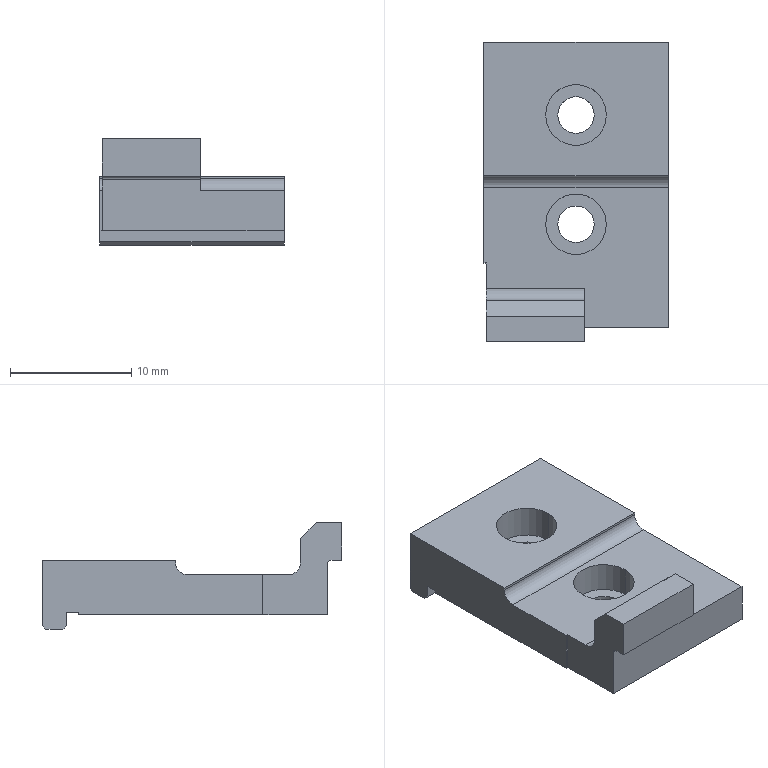Part | NX | 1 solid | 35 faces | box 15.2 x 24.7 x 8.8 mm | volume 1393 mm3 | plane 24 | cylinder 11 | commonest cylinder face diameters 3 x4 5 x4 2 x2 0.6 x1
STEP:
#1=CARTESIAN_POINT('',(0.2,6.5,-4.5));
#2=VERTEX_POINT('',#1);
#3=CARTESIAN_POINT('',(0.,6.5,-4.5));
#4=VERTEX_POINT('',#3);
#5=CARTESIAN_POINT('',(0.,6.5,-4.5));
#6=DIRECTION('',(-1.,0.,0.));
#7=VECTOR('',#6,1000.);
#8=LINE('',#5,#7);
#9=EDGE_CURVE('',#2,#4,#8,.T.);
#10=ORIENTED_EDGE('',*,*,#9,.T.);
#11=CARTESIAN_POINT('',(0.,21.7,-4.5));
#12=VERTEX_POINT('',#11);
#13=CARTESIAN_POINT('',(0.,0.,-4.5));
#14=DIRECTION('',(0.,-1.,0.));
#15=VECTOR('',#14,1000.);
#16=LINE('',#13,#15);
#17=EDGE_CURVE('',#12,#4,#16,.T.);
#18=ORIENTED_EDGE('',*,*,#17,.F.);
#19=CARTESIAN_POINT('',(15.2,21.7,-4.5));
#20=VERTEX_POINT('',#19);
#21=CARTESIAN_POINT('',(0.,21.7,-4.5));
#22=DIRECTION('',(1.,0.,0.));
#23=VECTOR('',#22,1000.);
#24=LINE('',#21,#23);
#25=EDGE_CURVE('',#12,#20,#24,.T.);
#26=ORIENTED_EDGE('',*,*,#25,.T.);
#27=CARTESIAN_POINT('',(15.2,1.2,-4.5));
#28=VERTEX_POINT('',#27);
#29=CARTESIAN_POINT('',(15.2,0.,-4.5));
#30=DIRECTION('',(0.,1.,0.));
#31=VECTOR('',#30,1000.);
#32=LINE('',#29,#31);
#33=EDGE_CURVE('',#28,#20,#32,.T.);
#34=ORIENTED_EDGE('',*,*,#33,.F.);
#35=CARTESIAN_POINT('',(0.2,1.2,-4.5));
#36=VERTEX_POINT('',#35);
#37=CARTESIAN_POINT('',(0.,1.2,-4.5));
#38=DIRECTION('',(-1.,0.,0.));
#39=VECTOR('',#38,1000.);
#40=LINE('',#37,#39);
#41=EDGE_CURVE('',#28,#36,#40,.T.);
#42=ORIENTED_EDGE('',*,*,#41,.T.);
#43=CARTESIAN_POINT('',(0.2,0.,-4.5));
#44=DIRECTION('',(0.,1.,0.));
#45=VECTOR('',#44,1000.);
#46=LINE('',#43,#45);
#47=EDGE_CURVE('',#36,#2,#46,.T.);
#48=ORIENTED_EDGE('',*,*,#47,.T.);
#49=EDGE_LOOP('',(#10,#18,#26,#34,#42,#48));
#50=FACE_BOUND('',#49,.T.);
#51=CARTESIAN_POINT('',(9.1,9.7,-4.5));
#52=VERTEX_POINT('',#51);
#53=CARTESIAN_POINT('',(6.1,9.7,-4.5));
#54=VERTEX_POINT('',#53);
#55=CARTESIAN_POINT('',(7.6,9.7,-4.5));
#56=DIRECTION('',(0.,0.,1.));
#57=DIRECTION('',(-1.,0.,0.));
#58=AXIS2_PLACEMENT_3D('',#55,#56,#57);
#59=CIRCLE('',#58,1.5);
#60=EDGE_CURVE('',#52,#54,#59,.T.);
#61=ORIENTED_EDGE('',*,*,#60,.T.);
#62=CARTESIAN_POINT('',(7.6,9.7,-4.5));
#63=DIRECTION('',(0.,0.,1.));
#64=DIRECTION('',(-1.,0.,0.));
#65=AXIS2_PLACEMENT_3D('',#62,#63,#64);
#66=CIRCLE('',#65,1.5);
#67=EDGE_CURVE('',#54,#52,#66,.T.);
#68=ORIENTED_EDGE('',*,*,#67,.T.);
#69=EDGE_LOOP('',(#61,#68));
#70=FACE_BOUND('',#69,.T.);
#71=CARTESIAN_POINT('',(6.1,18.7,-4.5));
#72=VERTEX_POINT('',#71);
#73=CARTESIAN_POINT('',(9.1,18.7,-4.5));
#74=VERTEX_POINT('',#73);
#75=CARTESIAN_POINT('',(7.6,18.7,-4.5));
#76=DIRECTION('',(0.,0.,1.));
#77=DIRECTION('',(-1.,0.,0.));
#78=AXIS2_PLACEMENT_3D('',#75,#76,#77);
#79=CIRCLE('',#78,1.5);
#80=EDGE_CURVE('',#72,#74,#79,.T.);
#81=ORIENTED_EDGE('',*,*,#80,.T.);
#82=CARTESIAN_POINT('',(7.6,18.7,-4.5));
#83=DIRECTION('',(0.,0.,1.));
#84=DIRECTION('',(-1.,0.,0.));
#85=AXIS2_PLACEMENT_3D('',#82,#83,#84);
#86=CIRCLE('',#85,1.5);
#87=EDGE_CURVE('',#74,#72,#86,.T.);
#88=ORIENTED_EDGE('',*,*,#87,.T.);
#89=EDGE_LOOP('',(#81,#88));
#90=FACE_BOUND('',#89,.T.);
#91=CARTESIAN_POINT('',(0.,0.,-4.5));
#92=DIRECTION('',(0.,0.,1.));
#93=DIRECTION('',(1.,0.,0.));
#94=AXIS2_PLACEMENT_3D('',#91,#92,#93);
#95=PLANE('',#94);
#96=ADVANCED_FACE('',(#50,#70,#90),#95,.F.);
#97=CARTESIAN_POINT('',(0.2,4.4,-1.2));
#98=VERTEX_POINT('',#97);
#99=CARTESIAN_POINT('',(0.2,6.5,-1.2));
#100=VERTEX_POINT('',#99);
#101=CARTESIAN_POINT('',(0.2,0.,-1.2));
#102=DIRECTION('',(0.,1.,0.));
#103=VECTOR('',#102,1000.);
#104=LINE('',#101,#103);
#105=EDGE_CURVE('',#98,#100,#104,.T.);
#106=ORIENTED_EDGE('',*,*,#105,.T.);
#107=CARTESIAN_POINT('',(0.2,6.5,0.));
#108=DIRECTION('',(0.,0.,-1.));
#109=VECTOR('',#108,1000.);
#110=LINE('',#107,#109);
#111=EDGE_CURVE('',#100,#2,#110,.T.);
#112=ORIENTED_EDGE('',*,*,#111,.T.);
#113=ORIENTED_EDGE('',*,*,#47,.F.);
#114=CARTESIAN_POINT('',(0.2,1.2,-0.3));
#115=VERTEX_POINT('',#114);
#116=CARTESIAN_POINT('',(0.2,1.2,0.));
#117=DIRECTION('',(0.,0.,-1.));
#118=VECTOR('',#117,1000.);
#119=LINE('',#116,#118);
#120=EDGE_CURVE('',#115,#36,#119,.T.);
#121=ORIENTED_EDGE('',*,*,#120,.F.);
#122=CARTESIAN_POINT('',(0.2,0.9,0.));
#123=VERTEX_POINT('',#122);
#124=CARTESIAN_POINT('',(0.2,0.9,-0.3));
#125=DIRECTION('',(-1.,0.,0.));
#126=DIRECTION('',(0.,0.,1.));
#127=AXIS2_PLACEMENT_3D('',#124,#125,#126);
#128=CIRCLE('',#127,0.3);
#129=EDGE_CURVE('',#123,#115,#128,.T.);
#130=ORIENTED_EDGE('',*,*,#129,.F.);
#131=CARTESIAN_POINT('',(0.2,0.,0.));
#132=VERTEX_POINT('',#131);
#133=CARTESIAN_POINT('',(0.2,0.,0.));
#134=DIRECTION('',(0.,1.,0.));
#135=VECTOR('',#134,1000.);
#136=LINE('',#133,#135);
#137=EDGE_CURVE('',#132,#123,#136,.T.);
#138=ORIENTED_EDGE('',*,*,#137,.F.);
#139=CARTESIAN_POINT('',(0.2,0.,3.1));
#140=VERTEX_POINT('',#139);
#141=CARTESIAN_POINT('',(0.2,0.,0.));
#142=DIRECTION('',(0.,0.,1.));
#143=VECTOR('',#142,1000.);
#144=LINE('',#141,#143);
#145=EDGE_CURVE('',#132,#140,#144,.T.);
#146=ORIENTED_EDGE('',*,*,#145,.T.);
#147=CARTESIAN_POINT('',(0.2,2.1,3.1));
#148=VERTEX_POINT('',#147);
#149=CARTESIAN_POINT('',(0.2,0.,3.1));
#150=DIRECTION('',(0.,1.,0.));
#151=VECTOR('',#150,1000.);
#152=LINE('',#149,#151);
#153=EDGE_CURVE('',#140,#148,#152,.T.);
#154=ORIENTED_EDGE('',*,*,#153,.T.);
#155=CARTESIAN_POINT('',(0.2,3.4,1.8));
#156=VERTEX_POINT('',#155);
#157=CARTESIAN_POINT('',(0.2,5.2,0.));
#158=DIRECTION('',(0.,-0.7071,0.7071));
#159=VECTOR('',#158,1000.);
#160=LINE('',#157,#159);
#161=EDGE_CURVE('',#156,#148,#160,.T.);
#162=ORIENTED_EDGE('',*,*,#161,.F.);
#163=CARTESIAN_POINT('',(0.2,3.4,-0.2));
#164=VERTEX_POINT('',#163);
#165=CARTESIAN_POINT('',(0.2,3.4,0.));
#166=DIRECTION('',(0.,0.,1.));
#167=VECTOR('',#166,1000.);
#168=LINE('',#165,#167);
#169=EDGE_CURVE('',#164,#156,#168,.T.);
#170=ORIENTED_EDGE('',*,*,#169,.F.);
#171=CARTESIAN_POINT('',(0.2,4.4,-0.2));
#172=DIRECTION('',(-1.,0.,0.));
#173=DIRECTION('',(0.,1.,0.));
#174=AXIS2_PLACEMENT_3D('',#171,#172,#173);
#175=CIRCLE('',#174,1.);
#176=EDGE_CURVE('',#98,#164,#175,.T.);
#177=ORIENTED_EDGE('',*,*,#176,.F.);
#178=EDGE_LOOP('',(#106,#112,#113,#121,#130,#138,#146,#154,#162,#170,#177));
#179=FACE_BOUND('',#178,.T.);
#180=CARTESIAN_POINT('',(0.2,6.5,-2.));
#181=DIRECTION('',(1.,0.,0.));
#182=DIRECTION('',(0.,1.,0.));
#183=AXIS2_PLACEMENT_3D('',#180,#181,#182);
#184=PLANE('',#183);
#185=ADVANCED_FACE('',(#179),#184,.F.);
#186=ORIENTED_EDGE('',*,*,#9,.F.);
#187=ORIENTED_EDGE('',*,*,#111,.F.);
#188=CARTESIAN_POINT('',(0.,6.5,-1.2));
#189=VERTEX_POINT('',#188);
#190=CARTESIAN_POINT('',(0.,6.5,-1.2));
#191=DIRECTION('',(1.,0.,0.));
#192=VECTOR('',#191,1000.);
#193=LINE('',#190,#192);
#194=EDGE_CURVE('',#189,#100,#193,.T.);
#195=ORIENTED_EDGE('',*,*,#194,.F.);
#196=CARTESIAN_POINT('',(0.,6.5,0.));
#197=DIRECTION('',(0.,0.,1.));
#198=VECTOR('',#197,1000.);
#199=LINE('',#196,#198);
#200=EDGE_CURVE('',#4,#189,#199,.T.);
#201=ORIENTED_EDGE('',*,*,#200,.F.);
#202=EDGE_LOOP('',(#186,#187,#195,#201));
#203=FACE_BOUND('',#202,.T.);
#204=CARTESIAN_POINT('',(0.,6.5,-2.));
#205=DIRECTION('',(0.,1.,0.));
#206=DIRECTION('',(1.,0.,0.));
#207=AXIS2_PLACEMENT_3D('',#204,#205,#206);
#208=PLANE('',#207);
#209=ADVANCED_FACE('',(#203),#208,.F.);
#210=CARTESIAN_POINT('',(10.1,18.7,-2.7));
#211=VERTEX_POINT('',#210);
#212=CARTESIAN_POINT('',(5.1,18.7,-2.7));
#213=VERTEX_POINT('',#212);
#214=CARTESIAN_POINT('',(7.6,18.7,-2.7));
#215=DIRECTION('',(0.,0.,1.));
#216=DIRECTION('',(-1.,0.,0.));
#217=AXIS2_PLACEMENT_3D('',#214,#215,#216);
#218=CIRCLE('',#217,2.5);
#219=EDGE_CURVE('',#211,#213,#218,.T.);
#220=ORIENTED_EDGE('',*,*,#219,.T.);
#221=CARTESIAN_POINT('',(7.6,18.7,-2.7));
#222=DIRECTION('',(0.,0.,1.));
#223=DIRECTION('',(-1.,0.,0.));
#224=AXIS2_PLACEMENT_3D('',#221,#222,#223);
#225=CIRCLE('',#224,2.5);
#226=EDGE_CURVE('',#213,#211,#225,.T.);
#227=ORIENTED_EDGE('',*,*,#226,.T.);
#228=EDGE_LOOP('',(#220,#227));
#229=FACE_BOUND('',#228,.T.);
#230=CARTESIAN_POINT('',(6.1,18.7,-2.7));
#231=VERTEX_POINT('',#230);
#232=CARTESIAN_POINT('',(9.1,18.7,-2.7));
#233=VERTEX_POINT('',#232);
#234=CARTESIAN_POINT('',(7.6,18.7,-2.7));
#235=DIRECTION('',(0.,0.,1.));
#236=DIRECTION('',(-1.,0.,0.));
#237=AXIS2_PLACEMENT_3D('',#234,#235,#236);
#238=CIRCLE('',#237,1.5);
#239=EDGE_CURVE('',#231,#233,#238,.T.);
#240=ORIENTED_EDGE('',*,*,#239,.F.);
#241=CARTESIAN_POINT('',(7.6,18.7,-2.7));
#242=DIRECTION('',(0.,0.,1.));
#243=DIRECTION('',(-1.,0.,0.));
#244=AXIS2_PLACEMENT_3D('',#241,#242,#243);
#245=CIRCLE('',#244,1.5);
#246=EDGE_CURVE('',#233,#231,#245,.T.);
#247=ORIENTED_EDGE('',*,*,#246,.F.);
#248=EDGE_LOOP('',(#240,#247));
#249=FACE_BOUND('',#248,.T.);
#250=CARTESIAN_POINT('',(6.068,11.447,-2.7));
#251=DIRECTION('',(0.,0.,1.));
#252=DIRECTION('',(1.,0.,0.));
#253=AXIS2_PLACEMENT_3D('',#250,#251,#252);
#254=PLANE('',#253);
#255=ADVANCED_FACE('',(#229,#249),#254,.T.);
#256=CARTESIAN_POINT('',(0.,13.7,-0.2));
#257=VERTEX_POINT('',#256);
#258=CARTESIAN_POINT('',(0.,13.7,0.));
#259=VERTEX_POINT('',#258);
#260=CARTESIAN_POINT('',(0.,13.7,0.));
#261=DIRECTION('',(0.,0.,1.));
#262=VECTOR('',#261,1000.);
#263=LINE('',#260,#262);
#264=EDGE_CURVE('',#257,#259,#263,.T.);
#265=ORIENTED_EDGE('',*,*,#264,.T.);
#266=CARTESIAN_POINT('',(0.,24.7,0.));
#267=VERTEX_POINT('',#266);
#268=CARTESIAN_POINT('',(0.,0.,0.));
#269=DIRECTION('',(0.,-1.,0.));
#270=VECTOR('',#269,1000.);
#271=LINE('',#268,#270);
#272=EDGE_CURVE('',#267,#259,#271,.T.);
#273=ORIENTED_EDGE('',*,*,#272,.F.);
#274=CARTESIAN_POINT('',(0.,24.7,-5.4));
#275=VERTEX_POINT('',#274);
#276=CARTESIAN_POINT('',(0.,24.7,0.));
#277=DIRECTION('',(0.,0.,-1.));
#278=VECTOR('',#277,1000.);
#279=LINE('',#276,#278);
#280=EDGE_CURVE('',#267,#275,#279,.T.);
#281=ORIENTED_EDGE('',*,*,#280,.T.);
#282=CARTESIAN_POINT('',(0.,24.4,-5.7));
#283=VERTEX_POINT('',#282);
#284=CARTESIAN_POINT('',(0.,0.,-30.1));
#285=DIRECTION('',(0.,-0.7071,-0.7071));
#286=VECTOR('',#285,1000.);
#287=LINE('',#284,#286);
#288=EDGE_CURVE('',#275,#283,#287,.T.);
#289=ORIENTED_EDGE('',*,*,#288,.T.);
#290=CARTESIAN_POINT('',(0.,23.,-5.7));
#291=VERTEX_POINT('',#290);
#292=CARTESIAN_POINT('',(0.,0.,-5.7));
#293=DIRECTION('',(0.,1.,0.));
#294=VECTOR('',#293,1000.);
#295=LINE('',#292,#294);
#296=EDGE_CURVE('',#291,#283,#295,.T.);
#297=ORIENTED_EDGE('',*,*,#296,.F.);
#298=CARTESIAN_POINT('',(0.,22.7,-5.4));
#299=VERTEX_POINT('',#298);
#300=CARTESIAN_POINT('',(0.,0.,17.3));
#301=DIRECTION('',(0.,-0.7071,0.7071));
#302=VECTOR('',#301,1000.);
#303=LINE('',#300,#302);
#304=EDGE_CURVE('',#291,#299,#303,.T.);
#305=ORIENTED_EDGE('',*,*,#304,.T.);
#306=CARTESIAN_POINT('',(0.,22.7,-4.3));
#307=VERTEX_POINT('',#306);
#308=CARTESIAN_POINT('',(0.,22.7,0.));
#309=DIRECTION('',(0.,0.,-1.));
#310=VECTOR('',#309,1000.);
#311=LINE('',#308,#310);
#312=EDGE_CURVE('',#307,#299,#311,.T.);
#313=ORIENTED_EDGE('',*,*,#312,.F.);
#314=CARTESIAN_POINT('',(0.,21.7,-4.3));
#315=VERTEX_POINT('',#314);
#316=CARTESIAN_POINT('',(0.,0.,-4.3));
#317=DIRECTION('',(0.,-1.,0.));
#318=VECTOR('',#317,1000.);
#319=LINE('',#316,#318);
#320=EDGE_CURVE('',#307,#315,#319,.T.);
#321=ORIENTED_EDGE('',*,*,#320,.T.);
#322=CARTESIAN_POINT('',(0.,21.7,0.));
#323=DIRECTION('',(0.,0.,-1.));
#324=VECTOR('',#323,1000.);
#325=LINE('',#322,#324);
#326=EDGE_CURVE('',#315,#12,#325,.T.);
#327=ORIENTED_EDGE('',*,*,#326,.T.);
#328=ORIENTED_EDGE('',*,*,#17,.T.);
#329=ORIENTED_EDGE('',*,*,#200,.T.);
#330=CARTESIAN_POINT('',(0.,12.7,-1.2));
#331=VERTEX_POINT('',#330);
#332=CARTESIAN_POINT('',(0.,0.,-1.2));
#333=DIRECTION('',(0.,-1.,0.));
#334=VECTOR('',#333,1000.);
#335=LINE('',#332,#334);
#336=EDGE_CURVE('',#331,#189,#335,.T.);
#337=ORIENTED_EDGE('',*,*,#336,.F.);
#338=CARTESIAN_POINT('',(0.,12.7,-0.2));
#339=DIRECTION('',(-1.,0.,0.));
#340=DIRECTION('',(0.,1.,0.));
#341=AXIS2_PLACEMENT_3D('',#338,#339,#340);
#342=CIRCLE('',#341,1.);
#343=EDGE_CURVE('',#257,#331,#342,.T.);
#344=ORIENTED_EDGE('',*,*,#343,.F.);
#345=EDGE_LOOP('',(#265,#273,#281,#289,#297,#305,#313,#321,#327,#328,#329,#337,#344));
#346=FACE_BOUND('',#345,.T.);
#347=CARTESIAN_POINT('',(0.,24.7,0.));
#348=DIRECTION('',(-1.,0.,0.));
#349=DIRECTION('',(0.,0.,1.));
#350=AXIS2_PLACEMENT_3D('',#347,#348,#349);
#351=PLANE('',#350);
#352=ADVANCED_FACE('',(#346),#351,.T.);
#353=CARTESIAN_POINT('',(8.3,4.4,-1.2));
#354=VERTEX_POINT('',#353);
#355=CARTESIAN_POINT('',(0.,4.4,-1.2));
#356=DIRECTION('',(-1.,0.,0.));
#357=VECTOR('',#356,1000.);
#358=LINE('',#355,#357);
#359=EDGE_CURVE('',#354,#98,#358,.T.);
#360=ORIENTED_EDGE('',*,*,#359,.T.);
#361=ORIENTED_EDGE('',*,*,#176,.T.);
#362=CARTESIAN_POINT('',(8.3,3.4,-0.2));
#363=VERTEX_POINT('',#362);
#364=CARTESIAN_POINT('',(0.,3.4,-0.2));
#365=DIRECTION('',(-1.,0.,0.));
#366=VECTOR('',#365,1000.);
#367=LINE('',#364,#366);
#368=EDGE_CURVE('',#363,#164,#367,.T.);
#369=ORIENTED_EDGE('',*,*,#368,.F.);
#370=CARTESIAN_POINT('',(8.3,4.4,-0.2));
#371=DIRECTION('',(-1.,0.,0.));
#372=DIRECTION('',(0.,1.,0.));
#373=AXIS2_PLACEMENT_3D('',#370,#371,#372);
#374=CIRCLE('',#373,1.);
#375=EDGE_CURVE('',#354,#363,#374,.T.);
#376=ORIENTED_EDGE('',*,*,#375,.F.);
#377=EDGE_LOOP('',(#360,#361,#369,#376));
#378=FACE_BOUND('',#377,.T.);
#379=CARTESIAN_POINT('',(0.,4.4,-0.2));
#380=DIRECTION('',(-1.,0.,0.));
#381=DIRECTION('',(0.,1.,0.));
#382=AXIS2_PLACEMENT_3D('',#379,#380,#381);
#383=CYLINDRICAL_SURFACE('',#382,1.);
#384=ADVANCED_FACE('',(#378),#383,.F.);
#385=ORIENTED_EDGE('',*,*,#264,.F.);
#386=CARTESIAN_POINT('',(15.2,13.7,-0.2));
#387=VERTEX_POINT('',#386);
#388=CARTESIAN_POINT('',(0.,13.7,-0.2));
#389=DIRECTION('',(-1.,0.,0.));
#390=VECTOR('',#389,1000.);
#391=LINE('',#388,#390);
#392=EDGE_CURVE('',#387,#257,#391,.T.);
#393=ORIENTED_EDGE('',*,*,#392,.F.);
#394=CARTESIAN_POINT('',(15.2,13.7,0.));
#395=VERTEX_POINT('',#394);
#396=CARTESIAN_POINT('',(15.2,13.7,0.));
#397=DIRECTION('',(0.,0.,-1.));
#398=VECTOR('',#397,1000.);
#399=LINE('',#396,#398);
#400=EDGE_CURVE('',#395,#387,#399,.T.);
#401=ORIENTED_EDGE('',*,*,#400,.F.);
#402=CARTESIAN_POINT('',(0.,13.7,0.));
#403=DIRECTION('',(-1.,0.,0.));
#404=VECTOR('',#403,1000.);
#405=LINE('',#402,#404);
#406=EDGE_CURVE('',#395,#259,#405,.T.);
#407=ORIENTED_EDGE('',*,*,#406,.T.);
#408=EDGE_LOOP('',(#385,#393,#401,#407));
#409=FACE_BOUND('',#408,.T.);
#410=CARTESIAN_POINT('',(15.2,13.7,-1.));
#411=DIRECTION('',(0.,1.,0.));
#412=DIRECTION('',(1.,0.,0.));
#413=AXIS2_PLACEMENT_3D('',#410,#411,#412);
#414=PLANE('',#413);
#415=ADVANCED_FACE('',(#409),#414,.F.);
#416=ORIENTED_EDGE('',*,*,#120,.T.);
#417=ORIENTED_EDGE('',*,*,#41,.F.);
#418=CARTESIAN_POINT('',(15.2,1.2,-1.2));
#419=VERTEX_POINT('',#418);
#420=CARTESIAN_POINT('',(15.2,1.2,0.));
#421=DIRECTION('',(0.,0.,-1.));
#422=VECTOR('',#421,1000.);
#423=LINE('',#420,#422);
#424=EDGE_CURVE('',#419,#28,#423,.T.);
#425=ORIENTED_EDGE('',*,*,#424,.F.);
#426=CARTESIAN_POINT('',(8.3,1.2,-1.2));
#427=VERTEX_POINT('',#426);
#428=CARTESIAN_POINT('',(0.,1.2,-1.2));
#429=DIRECTION('',(1.,0.,0.));
#430=VECTOR('',#429,1000.);
#431=LINE('',#428,#430);
#432=EDGE_CURVE('',#427,#419,#431,.T.);
#433=ORIENTED_EDGE('',*,*,#432,.F.);
#434=CARTESIAN_POINT('',(8.3,1.2,-0.3));
#435=VERTEX_POINT('',#434);
#436=CARTESIAN_POINT('',(8.3,1.2,0.));
#437=DIRECTION('',(0.,0.,1.));
#438=VECTOR('',#437,1000.);
#439=LINE('',#436,#438);
#440=EDGE_CURVE('',#427,#435,#439,.T.);
#441=ORIENTED_EDGE('',*,*,#440,.T.);
#442=CARTESIAN_POINT('',(15.289,1.2,-0.3));
#443=DIRECTION('',(-1.,0.,0.));
#444=VECTOR('',#443,1000.);
#445=LINE('',#442,#444);
#446=EDGE_CURVE('',#435,#115,#445,.T.);
#447=ORIENTED_EDGE('',*,*,#446,.T.);
#448=EDGE_LOOP('',(#416,#417,#425,#433,#441,#447));
#449=FACE_BOUND('',#448,.T.);
#450=CARTESIAN_POINT('',(15.2,1.2,-2.));
#451=DIRECTION('',(0.,1.,0.));
#452=DIRECTION('',(1.,0.,0.));
#453=AXIS2_PLACEMENT_3D('',#450,#451,#452);
#454=PLANE('',#453);
#455=ADVANCED_FACE('',(#449),#454,.F.);
#456=ORIENTED_EDGE('',*,*,#129,.T.);
#457=ORIENTED_EDGE('',*,*,#446,.F.);
#458=CARTESIAN_POINT('',(8.3,0.9,0.));
#459=VERTEX_POINT('',#458);
#460=CARTESIAN_POINT('',(8.3,0.9,-0.3));
#461=DIRECTION('',(-1.,0.,0.));
#462=DIRECTION('',(0.,0.,1.));
#463=AXIS2_PLACEMENT_3D('',#460,#461,#462);
#464=CIRCLE('',#463,0.3);
#465=EDGE_CURVE('',#459,#435,#464,.T.);
#466=ORIENTED_EDGE('',*,*,#465,.F.);
#467=CARTESIAN_POINT('',(15.289,0.9,0.));
#468=DIRECTION('',(-1.,0.,0.));
#469=VECTOR('',#468,1000.);
#470=LINE('',#467,#469);
#471=EDGE_CURVE('',#459,#123,#470,.T.);
#472=ORIENTED_EDGE('',*,*,#471,.T.);
#473=EDGE_LOOP('',(#456,#457,#466,#472));
#474=FACE_BOUND('',#473,.T.);
#475=CARTESIAN_POINT('',(15.289,0.9,-0.3));
#476=DIRECTION('',(-1.,0.,0.));
#477=DIRECTION('',(0.,0.,1.));
#478=AXIS2_PLACEMENT_3D('',#475,#476,#477);
#479=CYLINDRICAL_SURFACE('',#478,0.3);
#480=ADVANCED_FACE('',(#474),#479,.F.);
#481=ORIENTED_EDGE('',*,*,#137,.T.);
#482=ORIENTED_EDGE('',*,*,#471,.F.);
#483=CARTESIAN_POINT('',(8.3,0.,0.));
#484=VERTEX_POINT('',#483);
#485=CARTESIAN_POINT('',(8.3,0.,0.));
#486=DIRECTION('',(0.,-1.,0.));
#487=VECTOR('',#486,1000.);
#488=LINE('',#485,#487);
#489=EDGE_CURVE('',#459,#484,#488,.T.);
#490=ORIENTED_EDGE('',*,*,#489,.T.);
#491=CARTESIAN_POINT('',(0.,0.,0.));
#492=DIRECTION('',(1.,0.,0.));
#493=VECTOR('',#492,1000.);
#494=LINE('',#491,#493);
#495=EDGE_CURVE('',#132,#484,#494,.T.);
#496=ORIENTED_EDGE('',*,*,#495,.F.);
#497=EDGE_LOOP('',(#481,#482,#490,#496));
#498=FACE_BOUND('',#497,.T.);
#499=CARTESIAN_POINT('',(15.2,1.2,0.));
#500=DIRECTION('',(0.,0.,1.));
#501=DIRECTION('',(1.,0.,0.));
#502=AXIS2_PLACEMENT_3D('',#499,#500,#501);
#503=PLANE('',#502);
#504=ADVANCED_FACE('',(#498),#503,.F.);
#505=ORIENTED_EDGE('',*,*,#145,.F.);
#506=ORIENTED_EDGE('',*,*,#495,.T.);
#507=CARTESIAN_POINT('',(8.3,0.,3.1));
#508=VERTEX_POINT('',#507);
#509=CARTESIAN_POINT('',(8.3,0.,0.));
#510=DIRECTION('',(0.,0.,1.));
#511=VECTOR('',#510,1000.);
#512=LINE('',#509,#511);
#513=EDGE_CURVE('',#484,#508,#512,.T.);
#514=ORIENTED_EDGE('',*,*,#513,.T.);
#515=CARTESIAN_POINT('',(0.,0.,3.1));
#516=DIRECTION('',(-1.,0.,0.));
#517=VECTOR('',#516,1000.);
#518=LINE('',#515,#517);
#519=EDGE_CURVE('',#508,#140,#518,.T.);
#520=ORIENTED_EDGE('',*,*,#519,.T.);
#521=EDGE_LOOP('',(#505,#506,#514,#520));
#522=FACE_BOUND('',#521,.T.);
#523=CARTESIAN_POINT('',(0.,0.,0.));
#524=DIRECTION('',(0.,-1.,0.));
#525=DIRECTION('',(0.,0.,-1.));
#526=AXIS2_PLACEMENT_3D('',#523,#524,#525);
#527=PLANE('',#526);
#528=ADVANCED_FACE('',(#522),#527,.T.);
#529=ORIENTED_EDGE('',*,*,#153,.F.);
#530=ORIENTED_EDGE('',*,*,#519,.F.);
#531=CARTESIAN_POINT('',(8.3,2.1,3.1));
#532=VERTEX_POINT('',#531);
#533=CARTESIAN_POINT('',(8.3,0.,3.1));
#534=DIRECTION('',(0.,1.,0.));
#535=VECTOR('',#534,1000.);
#536=LINE('',#533,#535);
#537=EDGE_CURVE('',#508,#532,#536,.T.);
#538=ORIENTED_EDGE('',*,*,#537,.T.);
#539=CARTESIAN_POINT('',(0.,2.1,3.1));
#540=DIRECTION('',(-1.,0.,0.));
#541=VECTOR('',#540,1000.);
#542=LINE('',#539,#541);
#543=EDGE_CURVE('',#532,#148,#542,.T.);
#544=ORIENTED_EDGE('',*,*,#543,.T.);
#545=EDGE_LOOP('',(#529,#530,#538,#544));
#546=FACE_BOUND('',#545,.T.);
#547=CARTESIAN_POINT('',(0.,0.,3.1));
#548=DIRECTION('',(0.,0.,1.));
#549=DIRECTION('',(1.,0.,0.));
#550=AXIS2_PLACEMENT_3D('',#547,#548,#549);
#551=PLANE('',#550);
#552=ADVANCED_FACE('',(#546),#551,.T.);
#553=ORIENTED_EDGE('',*,*,#161,.T.);
#554=ORIENTED_EDGE('',*,*,#543,.F.);
#555=CARTESIAN_POINT('',(8.3,3.4,1.8));
#556=VERTEX_POINT('',#555);
#557=CARTESIAN_POINT('',(8.3,5.2,0.));
#558=DIRECTION('',(0.,-0.7071,0.7071));
#559=VECTOR('',#558,1000.);
#560=LINE('',#557,#559);
#561=EDGE_CURVE('',#556,#532,#560,.T.);
#562=ORIENTED_EDGE('',*,*,#561,.F.);
#563=CARTESIAN_POINT('',(0.,3.4,1.8));
#564=DIRECTION('',(1.,0.,0.));
#565=VECTOR('',#564,1000.);
#566=LINE('',#563,#565);
#567=EDGE_CURVE('',#156,#556,#566,.T.);
#568=ORIENTED_EDGE('',*,*,#567,.F.);
#569=EDGE_LOOP('',(#553,#554,#562,#568));
#570=FACE_BOUND('',#569,.T.);
#571=CARTESIAN_POINT('',(15.2,2.4,2.8));
#572=DIRECTION('',(0.,-0.7071,-0.7071));
#573=DIRECTION('',(0.,-0.7071,0.7071));
#574=AXIS2_PLACEMENT_3D('',#571,#572,#573);
#575=PLANE('',#574);
#576=ADVANCED_FACE('',(#570),#575,.F.);
#577=CARTESIAN_POINT('',(8.3,3.4,0.));
#578=DIRECTION('',(0.,0.,-1.));
#579=VECTOR('',#578,1000.);
#580=LINE('',#577,#579);
#581=EDGE_CURVE('',#556,#363,#580,.T.);
#582=ORIENTED_EDGE('',*,*,#581,.T.);
#583=ORIENTED_EDGE('',*,*,#368,.T.);
#584=ORIENTED_EDGE('',*,*,#169,.T.);
#585=ORIENTED_EDGE('',*,*,#567,.T.);
#586=EDGE_LOOP('',(#582,#583,#584,#585));
#587=FACE_BOUND('',#586,.T.);
#588=CARTESIAN_POINT('',(0.2,3.4,-1.));
#589=DIRECTION('',(0.,-1.,0.));
#590=DIRECTION('',(0.,0.,-1.));
#591=AXIS2_PLACEMENT_3D('',#588,#589,#590);
#592=PLANE('',#591);
#593=ADVANCED_FACE('',(#587),#592,.F.);
#594=ORIENTED_EDGE('',*,*,#400,.T.);
#595=CARTESIAN_POINT('',(15.2,12.7,-1.2));
#596=VERTEX_POINT('',#595);
#597=CARTESIAN_POINT('',(15.2,12.7,-0.2));
#598=DIRECTION('',(-1.,0.,0.));
#599=DIRECTION('',(0.,1.,0.));
#600=AXIS2_PLACEMENT_3D('',#597,#598,#599);
#601=CIRCLE('',#600,1.);
#602=EDGE_CURVE('',#387,#596,#601,.T.);
#603=ORIENTED_EDGE('',*,*,#602,.T.);
#604=CARTESIAN_POINT('',(15.2,0.,-1.2));
#605=DIRECTION('',(0.,1.,0.));
#606=VECTOR('',#605,1000.);
#607=LINE('',#604,#606);
#608=EDGE_CURVE('',#419,#596,#607,.T.);
#609=ORIENTED_EDGE('',*,*,#608,.F.);
#610=ORIENTED_EDGE('',*,*,#424,.T.);
#611=ORIENTED_EDGE('',*,*,#33,.T.);
#612=CARTESIAN_POINT('',(15.2,21.7,-4.3));
#613=VERTEX_POINT('',#612);
#614=CARTESIAN_POINT('',(15.2,21.7,0.));
#615=DIRECTION('',(0.,0.,1.));
#616=VECTOR('',#615,1000.);
#617=LINE('',#614,#616);
#618=EDGE_CURVE('',#20,#613,#617,.T.);
#619=ORIENTED_EDGE('',*,*,#618,.T.);
#620=CARTESIAN_POINT('',(15.2,22.7,-4.3));
#621=VERTEX_POINT('',#620);
#622=CARTESIAN_POINT('',(15.2,0.,-4.3));
#623=DIRECTION('',(0.,1.,0.));
#624=VECTOR('',#623,1000.);
#625=LINE('',#622,#624);
#626=EDGE_CURVE('',#613,#621,#625,.T.);
#627=ORIENTED_EDGE('',*,*,#626,.T.);
#628=CARTESIAN_POINT('',(15.2,22.7,-5.4));
#629=VERTEX_POINT('',#628);
#630=CARTESIAN_POINT('',(15.2,22.7,0.));
#631=DIRECTION('',(0.,0.,1.));
#632=VECTOR('',#631,1000.);
#633=LINE('',#630,#632);
#634=EDGE_CURVE('',#629,#621,#633,.T.);
#635=ORIENTED_EDGE('',*,*,#634,.F.);
#636=CARTESIAN_POINT('',(15.2,23.,-5.7));
#637=VERTEX_POINT('',#636);
#638=CARTESIAN_POINT('',(15.2,0.,17.3));
#639=DIRECTION('',(0.,0.7071,-0.7071));
#640=VECTOR('',#639,1000.);
#641=LINE('',#638,#640);
#642=EDGE_CURVE('',#629,#637,#641,.T.);
#643=ORIENTED_EDGE('',*,*,#642,.T.);
#644=CARTESIAN_POINT('',(15.2,24.4,-5.7));
#645=VERTEX_POINT('',#644);
#646=CARTESIAN_POINT('',(15.2,0.,-5.7));
#647=DIRECTION('',(0.,-1.,0.));
#648=VECTOR('',#647,1000.);
#649=LINE('',#646,#648);
#650=EDGE_CURVE('',#645,#637,#649,.T.);
#651=ORIENTED_EDGE('',*,*,#650,.F.);
#652=CARTESIAN_POINT('',(15.2,24.7,-5.4));
#653=VERTEX_POINT('',#652);
#654=CARTESIAN_POINT('',(15.2,0.,-30.1));
#655=DIRECTION('',(0.,0.7071,0.7071));
#656=VECTOR('',#655,1000.);
#657=LINE('',#654,#656);
#658=EDGE_CURVE('',#645,#653,#657,.T.);
#659=ORIENTED_EDGE('',*,*,#658,.T.);
#660=CARTESIAN_POINT('',(15.2,24.7,0.));
#661=VERTEX_POINT('',#660);
#662=CARTESIAN_POINT('',(15.2,24.7,0.));
#663=DIRECTION('',(0.,0.,-1.));
#664=VECTOR('',#663,1000.);
#665=LINE('',#662,#664);
#666=EDGE_CURVE('',#661,#653,#665,.T.);
#667=ORIENTED_EDGE('',*,*,#666,.F.);
#668=CARTESIAN_POINT('',(15.2,0.,0.));
#669=DIRECTION('',(0.,1.,0.));
#670=VECTOR('',#669,1000.);
#671=LINE('',#668,#670);
#672=EDGE_CURVE('',#395,#661,#671,.T.);
#673=ORIENTED_EDGE('',*,*,#672,.F.);
#674=EDGE_LOOP('',(#594,#603,#609,#610,#611,#619,#627,#635,#643,#651,#659,#667,#673));
#675=FACE_BOUND('',#674,.T.);
#676=CARTESIAN_POINT('',(15.2,0.,0.));
#677=DIRECTION('',(1.,0.,0.));
#678=DIRECTION('',(0.,1.,0.));
#679=AXIS2_PLACEMENT_3D('',#676,#677,#678);
#680=PLANE('',#679);
#681=ADVANCED_FACE('',(#675),#680,.T.);
#682=CARTESIAN_POINT('',(0.,24.7,-5.4));
#683=DIRECTION('',(-1.,0.,0.));
#684=VECTOR('',#683,1000.);
#685=LINE('',#682,#684);
#686=EDGE_CURVE('',#653,#275,#685,.T.);
#687=ORIENTED_EDGE('',*,*,#686,.T.);
#688=ORIENTED_EDGE('',*,*,#280,.F.);
#689=CARTESIAN_POINT('',(0.,24.7,0.));
#690=DIRECTION('',(-1.,0.,0.));
#691=VECTOR('',#690,1000.);
#692=LINE('',#689,#691);
#693=EDGE_CURVE('',#661,#267,#692,.T.);
#694=ORIENTED_EDGE('',*,*,#693,.F.);
#695=ORIENTED_EDGE('',*,*,#666,.T.);
#696=EDGE_LOOP('',(#687,#688,#694,#695));
#697=FACE_BOUND('',#696,.T.);
#698=CARTESIAN_POINT('',(15.2,24.7,0.));
#699=DIRECTION('',(0.,1.,0.));
#700=DIRECTION('',(1.,0.,0.));
#701=AXIS2_PLACEMENT_3D('',#698,#699,#700);
#702=PLANE('',#701);
#703=ADVANCED_FACE('',(#697),#702,.T.);
#704=CARTESIAN_POINT('',(0.,23.,-5.7));
#705=DIRECTION('',(-1.,0.,0.));
#706=VECTOR('',#705,1000.);
#707=LINE('',#704,#706);
#708=EDGE_CURVE('',#637,#291,#707,.T.);
#709=ORIENTED_EDGE('',*,*,#708,.T.);
#710=ORIENTED_EDGE('',*,*,#296,.T.);
#711=CARTESIAN_POINT('',(0.,24.4,-5.7));
#712=DIRECTION('',(1.,0.,0.));
#713=VECTOR('',#712,1000.);
#714=LINE('',#711,#713);
#715=EDGE_CURVE('',#283,#645,#714,.T.);
#716=ORIENTED_EDGE('',*,*,#715,.T.);
#717=ORIENTED_EDGE('',*,*,#650,.T.);
#718=EDGE_LOOP('',(#709,#710,#716,#717));
#719=FACE_BOUND('',#718,.T.);
#720=CARTESIAN_POINT('',(0.,22.7,-5.7));
#721=DIRECTION('',(0.,0.,-1.));
#722=DIRECTION('',(0.,-1.,0.));
#723=AXIS2_PLACEMENT_3D('',#720,#721,#722);
#724=PLANE('',#723);
#725=ADVANCED_FACE('',(#719),#724,.T.);
#726=ORIENTED_EDGE('',*,*,#312,.T.);
#727=CARTESIAN_POINT('',(0.,22.7,-5.4));
#728=DIRECTION('',(1.,0.,0.));
#729=VECTOR('',#728,1000.);
#730=LINE('',#727,#729);
#731=EDGE_CURVE('',#299,#629,#730,.T.);
#732=ORIENTED_EDGE('',*,*,#731,.T.);
#733=ORIENTED_EDGE('',*,*,#634,.T.);
#734=CARTESIAN_POINT('',(0.,22.7,-4.3));
#735=DIRECTION('',(1.,0.,0.));
#736=VECTOR('',#735,1000.);
#737=LINE('',#734,#736);
#738=EDGE_CURVE('',#307,#621,#737,.T.);
#739=ORIENTED_EDGE('',*,*,#738,.F.);
#740=EDGE_LOOP('',(#726,#732,#733,#739));
#741=FACE_BOUND('',#740,.T.);
#742=CARTESIAN_POINT('',(0.,22.7,-2.));
#743=DIRECTION('',(0.,-1.,0.));
#744=DIRECTION('',(0.,0.,-1.));
#745=AXIS2_PLACEMENT_3D('',#742,#743,#744);
#746=PLANE('',#745);
#747=ADVANCED_FACE('',(#741),#746,.T.);
#748=ORIENTED_EDGE('',*,*,#626,.F.);
#749=CARTESIAN_POINT('',(0.,21.7,-4.3));
#750=DIRECTION('',(1.,0.,0.));
#751=VECTOR('',#750,1000.);
#752=LINE('',#749,#751);
#753=EDGE_CURVE('',#315,#613,#752,.T.);
#754=ORIENTED_EDGE('',*,*,#753,.F.);
#755=ORIENTED_EDGE('',*,*,#320,.F.);
#756=ORIENTED_EDGE('',*,*,#738,.T.);
#757=EDGE_LOOP('',(#748,#754,#755,#756));
#758=FACE_BOUND('',#757,.T.);
#759=CARTESIAN_POINT('',(0.,21.7,-4.3));
#760=DIRECTION('',(0.,0.,1.));
#761=DIRECTION('',(1.,0.,0.));
#762=AXIS2_PLACEMENT_3D('',#759,#760,#761);
#763=PLANE('',#762);
#764=ADVANCED_FACE('',(#758),#763,.F.);
#765=ORIENTED_EDGE('',*,*,#25,.F.);
#766=ORIENTED_EDGE('',*,*,#326,.F.);
#767=ORIENTED_EDGE('',*,*,#753,.T.);
#768=ORIENTED_EDGE('',*,*,#618,.F.);
#769=EDGE_LOOP('',(#765,#766,#767,#768));
#770=FACE_BOUND('',#769,.T.);
#771=CARTESIAN_POINT('',(0.,21.7,-2.));
#772=DIRECTION('',(0.,-1.,0.));
#773=DIRECTION('',(0.,0.,-1.));
#774=AXIS2_PLACEMENT_3D('',#771,#772,#773);
#775=PLANE('',#774);
#776=ADVANCED_FACE('',(#770),#775,.F.);
#777=ORIENTED_EDGE('',*,*,#60,.F.);
#778=CARTESIAN_POINT('',(9.1,9.7,-3.7));
#779=VERTEX_POINT('',#778);
#780=CARTESIAN_POINT('',(9.1,9.7,-5.23));
#781=DIRECTION('',(0.,0.,1.));
#782=VECTOR('',#781,1000.);
#783=LINE('',#780,#782);
#784=EDGE_CURVE('',#779,#52,#783,.F.);
#785=ORIENTED_EDGE('',*,*,#784,.F.);
#786=CARTESIAN_POINT('',(6.1,9.7,-3.7));
#787=VERTEX_POINT('',#786);
#788=CARTESIAN_POINT('',(7.6,9.7,-3.7));
#789=DIRECTION('',(0.,0.,1.));
#790=DIRECTION('',(-1.,0.,0.));
#791=AXIS2_PLACEMENT_3D('',#788,#789,#790);
#792=CIRCLE('',#791,1.5);
#793=EDGE_CURVE('',#779,#787,#792,.T.);
#794=ORIENTED_EDGE('',*,*,#793,.T.);
#795=CARTESIAN_POINT('',(6.1,9.7,-5.23));
#796=DIRECTION('',(0.,0.,1.));
#797=VECTOR('',#796,1000.);
#798=LINE('',#795,#797);
#799=EDGE_CURVE('',#787,#54,#798,.F.);
#800=ORIENTED_EDGE('',*,*,#799,.T.);
#801=EDGE_LOOP('',(#777,#785,#794,#800));
#802=FACE_BOUND('',#801,.T.);
#803=CARTESIAN_POINT('',(7.6,9.7,-5.23));
#804=DIRECTION('',(0.,0.,1.));
#805=DIRECTION('',(-1.,0.,0.));
#806=AXIS2_PLACEMENT_3D('',#803,#804,#805);
#807=CYLINDRICAL_SURFACE('',#806,1.5);
#808=ADVANCED_FACE('',(#802),#807,.F.);
#809=ORIENTED_EDGE('',*,*,#239,.T.);
#810=CARTESIAN_POINT('',(9.1,18.7,-5.23));
#811=DIRECTION('',(0.,0.,1.));
#812=VECTOR('',#811,1000.);
#813=LINE('',#810,#812);
#814=EDGE_CURVE('',#233,#74,#813,.F.);
#815=ORIENTED_EDGE('',*,*,#814,.T.);
#816=ORIENTED_EDGE('',*,*,#80,.F.);
#817=CARTESIAN_POINT('',(6.1,18.7,-5.23));
#818=DIRECTION('',(0.,0.,1.));
#819=VECTOR('',#818,1000.);
#820=LINE('',#817,#819);
#821=EDGE_CURVE('',#231,#72,#820,.F.);
#822=ORIENTED_EDGE('',*,*,#821,.F.);
#823=EDGE_LOOP('',(#809,#815,#816,#822));
#824=FACE_BOUND('',#823,.T.);
#825=CARTESIAN_POINT('',(7.6,18.7,-5.23));
#826=DIRECTION('',(0.,0.,1.));
#827=DIRECTION('',(-1.,0.,0.));
#828=AXIS2_PLACEMENT_3D('',#825,#826,#827);
#829=CYLINDRICAL_SURFACE('',#828,1.5);
#830=ADVANCED_FACE('',(#824),#829,.F.);
#831=CARTESIAN_POINT('',(5.1,9.7,-3.7));
#832=VERTEX_POINT('',#831);
#833=CARTESIAN_POINT('',(10.1,9.7,-3.7));
#834=VERTEX_POINT('',#833);
#835=CARTESIAN_POINT('',(7.6,9.7,-3.7));
#836=DIRECTION('',(0.,0.,1.));
#837=DIRECTION('',(-1.,0.,0.));
#838=AXIS2_PLACEMENT_3D('',#835,#836,#837);
#839=CIRCLE('',#838,2.5);
#840=EDGE_CURVE('',#832,#834,#839,.T.);
#841=ORIENTED_EDGE('',*,*,#840,.T.);
#842=CARTESIAN_POINT('',(7.6,9.7,-3.7));
#843=DIRECTION('',(0.,0.,1.));
#844=DIRECTION('',(-1.,0.,0.));
#845=AXIS2_PLACEMENT_3D('',#842,#843,#844);
#846=CIRCLE('',#845,2.5);
#847=EDGE_CURVE('',#834,#832,#846,.T.);
#848=ORIENTED_EDGE('',*,*,#847,.T.);
#849=EDGE_LOOP('',(#841,#848));
#850=FACE_BOUND('',#849,.T.);
#851=ORIENTED_EDGE('',*,*,#793,.F.);
#852=CARTESIAN_POINT('',(7.6,9.7,-3.7));
#853=DIRECTION('',(0.,0.,1.));
#854=DIRECTION('',(-1.,0.,0.));
#855=AXIS2_PLACEMENT_3D('',#852,#853,#854);
#856=CIRCLE('',#855,1.5);
#857=EDGE_CURVE('',#787,#779,#856,.T.);
#858=ORIENTED_EDGE('',*,*,#857,.F.);
#859=EDGE_LOOP('',(#851,#858));
#860=FACE_BOUND('',#859,.T.);
#861=CARTESIAN_POINT('',(6.068,11.447,-3.7));
#862=DIRECTION('',(0.,0.,1.));
#863=DIRECTION('',(1.,0.,0.));
#864=AXIS2_PLACEMENT_3D('',#861,#862,#863);
#865=PLANE('',#864);
#866=ADVANCED_FACE('',(#850,#860),#865,.T.);
#867=CARTESIAN_POINT('',(5.1,9.7,-1.2));
#868=VERTEX_POINT('',#867);
#869=CARTESIAN_POINT('',(10.1,9.7,-1.2));
#870=VERTEX_POINT('',#869);
#871=CARTESIAN_POINT('',(7.6,9.7,-1.2));
#872=DIRECTION('',(0.,0.,1.));
#873=DIRECTION('',(-1.,0.,0.));
#874=AXIS2_PLACEMENT_3D('',#871,#872,#873);
#875=CIRCLE('',#874,2.5);
#876=EDGE_CURVE('',#868,#870,#875,.T.);
#877=ORIENTED_EDGE('',*,*,#876,.T.);
#878=CARTESIAN_POINT('',(10.1,9.7,0.));
#879=DIRECTION('',(0.,0.,1.));
#880=VECTOR('',#879,1000.);
#881=LINE('',#878,#880);
#882=EDGE_CURVE('',#870,#834,#881,.F.);
#883=ORIENTED_EDGE('',*,*,#882,.T.);
#884=ORIENTED_EDGE('',*,*,#840,.F.);
#885=CARTESIAN_POINT('',(5.1,9.7,0.));
#886=DIRECTION('',(0.,0.,1.));
#887=VECTOR('',#886,1000.);
#888=LINE('',#885,#887);
#889=EDGE_CURVE('',#868,#832,#888,.F.);
#890=ORIENTED_EDGE('',*,*,#889,.F.);
#891=EDGE_LOOP('',(#877,#883,#884,#890));
#892=FACE_BOUND('',#891,.T.);
#893=CARTESIAN_POINT('',(7.6,9.7,0.));
#894=DIRECTION('',(0.,0.,1.));
#895=DIRECTION('',(-1.,0.,0.));
#896=AXIS2_PLACEMENT_3D('',#893,#894,#895);
#897=CYLINDRICAL_SURFACE('',#896,2.5);
#898=ADVANCED_FACE('',(#892),#897,.F.);
#899=ORIENTED_EDGE('',*,*,#406,.F.);
#900=ORIENTED_EDGE('',*,*,#672,.T.);
#901=ORIENTED_EDGE('',*,*,#693,.T.);
#902=ORIENTED_EDGE('',*,*,#272,.T.);
#903=EDGE_LOOP('',(#899,#900,#901,#902));
#904=FACE_BOUND('',#903,.T.);
#905=CARTESIAN_POINT('',(5.1,18.7,0.));
#906=VERTEX_POINT('',#905);
#907=CARTESIAN_POINT('',(10.1,18.7,0.));
#908=VERTEX_POINT('',#907);
#909=CARTESIAN_POINT('',(7.6,18.7,0.));
#910=DIRECTION('',(0.,0.,1.));
#911=DIRECTION('',(-1.,0.,0.));
#912=AXIS2_PLACEMENT_3D('',#909,#910,#911);
#913=CIRCLE('',#912,2.5);
#914=EDGE_CURVE('',#906,#908,#913,.T.);
#915=ORIENTED_EDGE('',*,*,#914,.F.);
#916=CARTESIAN_POINT('',(7.6,18.7,0.));
#917=DIRECTION('',(0.,0.,1.));
#918=DIRECTION('',(-1.,0.,0.));
#919=AXIS2_PLACEMENT_3D('',#916,#917,#918);
#920=CIRCLE('',#919,2.5);
#921=EDGE_CURVE('',#908,#906,#920,.T.);
#922=ORIENTED_EDGE('',*,*,#921,.F.);
#923=EDGE_LOOP('',(#915,#922));
#924=FACE_BOUND('',#923,.T.);
#925=CARTESIAN_POINT('',(0.,0.,0.));
#926=DIRECTION('',(0.,0.,1.));
#927=DIRECTION('',(1.,0.,0.));
#928=AXIS2_PLACEMENT_3D('',#925,#926,#927);
#929=PLANE('',#928);
#930=ADVANCED_FACE('',(#904,#924),#929,.T.);
#931=ORIENTED_EDGE('',*,*,#219,.F.);
#932=CARTESIAN_POINT('',(10.1,18.7,0.));
#933=DIRECTION('',(0.,0.,1.));
#934=VECTOR('',#933,1000.);
#935=LINE('',#932,#934);
#936=EDGE_CURVE('',#211,#908,#935,.T.);
#937=ORIENTED_EDGE('',*,*,#936,.T.);
#938=ORIENTED_EDGE('',*,*,#921,.T.);
#939=CARTESIAN_POINT('',(5.1,18.7,0.));
#940=DIRECTION('',(0.,0.,1.));
#941=VECTOR('',#940,1000.);
#942=LINE('',#939,#941);
#943=EDGE_CURVE('',#213,#906,#942,.T.);
#944=ORIENTED_EDGE('',*,*,#943,.F.);
#945=EDGE_LOOP('',(#931,#937,#938,#944));
#946=FACE_BOUND('',#945,.T.);
#947=CARTESIAN_POINT('',(7.6,18.7,0.));
#948=DIRECTION('',(0.,0.,1.));
#949=DIRECTION('',(-1.,0.,0.));
#950=AXIS2_PLACEMENT_3D('',#947,#948,#949);
#951=CYLINDRICAL_SURFACE('',#950,2.5);
#952=ADVANCED_FACE('',(#946),#951,.F.);
#953=CARTESIAN_POINT('',(0.,12.7,-1.2));
#954=DIRECTION('',(-1.,0.,0.));
#955=VECTOR('',#954,1000.);
#956=LINE('',#953,#955);
#957=EDGE_CURVE('',#596,#331,#956,.T.);
#958=ORIENTED_EDGE('',*,*,#957,.F.);
#959=ORIENTED_EDGE('',*,*,#602,.F.);
#960=ORIENTED_EDGE('',*,*,#392,.T.);
#961=ORIENTED_EDGE('',*,*,#343,.T.);
#962=EDGE_LOOP('',(#958,#959,#960,#961));
#963=FACE_BOUND('',#962,.T.);
#964=CARTESIAN_POINT('',(0.,12.7,-0.2));
#965=DIRECTION('',(-1.,0.,0.));
#966=DIRECTION('',(0.,1.,0.));
#967=AXIS2_PLACEMENT_3D('',#964,#965,#966);
#968=CYLINDRICAL_SURFACE('',#967,1.);
#969=ADVANCED_FACE('',(#963),#968,.F.);
#970=ORIENTED_EDGE('',*,*,#440,.F.);
#971=CARTESIAN_POINT('',(8.3,0.,-1.2));
#972=DIRECTION('',(0.,-1.,0.));
#973=VECTOR('',#972,1000.);
#974=LINE('',#971,#973);
#975=EDGE_CURVE('',#354,#427,#974,.T.);
#976=ORIENTED_EDGE('',*,*,#975,.F.);
#977=ORIENTED_EDGE('',*,*,#375,.T.);
#978=ORIENTED_EDGE('',*,*,#581,.F.);
#979=ORIENTED_EDGE('',*,*,#561,.T.);
#980=ORIENTED_EDGE('',*,*,#537,.F.);
#981=ORIENTED_EDGE('',*,*,#513,.F.);
#982=ORIENTED_EDGE('',*,*,#489,.F.);
#983=ORIENTED_EDGE('',*,*,#465,.T.);
#984=EDGE_LOOP('',(#970,#976,#977,#978,#979,#980,#981,#982,#983));
#985=FACE_BOUND('',#984,.T.);
#986=CARTESIAN_POINT('',(8.3,3.4,-1.));
#987=DIRECTION('',(-1.,0.,0.));
#988=DIRECTION('',(0.,0.,1.));
#989=AXIS2_PLACEMENT_3D('',#986,#987,#988);
#990=PLANE('',#989);
#991=ADVANCED_FACE('',(#985),#990,.F.);
#992=ORIENTED_EDGE('',*,*,#957,.T.);
#993=ORIENTED_EDGE('',*,*,#336,.T.);
#994=ORIENTED_EDGE('',*,*,#194,.T.);
#995=ORIENTED_EDGE('',*,*,#105,.F.);
#996=ORIENTED_EDGE('',*,*,#359,.F.);
#997=ORIENTED_EDGE('',*,*,#975,.T.);
#998=ORIENTED_EDGE('',*,*,#432,.T.);
#999=ORIENTED_EDGE('',*,*,#608,.T.);
#1000=EDGE_LOOP('',(#992,#993,#994,#995,#996,#997,#998,#999));
#1001=FACE_BOUND('',#1000,.T.);
#1002=ORIENTED_EDGE('',*,*,#876,.F.);
#1003=CARTESIAN_POINT('',(7.6,9.7,-1.2));
#1004=DIRECTION('',(0.,0.,1.));
#1005=DIRECTION('',(-1.,0.,0.));
#1006=AXIS2_PLACEMENT_3D('',#1003,#1004,#1005);
#1007=CIRCLE('',#1006,2.5);
#1008=EDGE_CURVE('',#870,#868,#1007,.T.);
#1009=ORIENTED_EDGE('',*,*,#1008,.F.);
#1010=EDGE_LOOP('',(#1002,#1009));
#1011=FACE_BOUND('',#1010,.T.);
#1012=CARTESIAN_POINT('',(10.928,7.264,-1.2));
#1013=DIRECTION('',(0.,0.,1.));
#1014=DIRECTION('',(1.,0.,0.));
#1015=AXIS2_PLACEMENT_3D('',#1012,#1013,#1014);
#1016=PLANE('',#1015);
#1017=ADVANCED_FACE('',(#1001,#1011),#1016,.T.);
#1018=ORIENTED_EDGE('',*,*,#686,.F.);
#1019=ORIENTED_EDGE('',*,*,#658,.F.);
#1020=ORIENTED_EDGE('',*,*,#715,.F.);
#1021=ORIENTED_EDGE('',*,*,#288,.F.);
#1022=EDGE_LOOP('',(#1018,#1019,#1020,#1021));
#1023=FACE_BOUND('',#1022,.T.);
#1024=CARTESIAN_POINT('',(7.6,24.55,-5.55));
#1025=DIRECTION('',(0.,-0.7071,0.7071));
#1026=DIRECTION('',(-1.,0.,0.));
#1027=AXIS2_PLACEMENT_3D('',#1024,#1025,#1026);
#1028=PLANE('',#1027);
#1029=ADVANCED_FACE('',(#1023),#1028,.F.);
#1030=ORIENTED_EDGE('',*,*,#708,.F.);
#1031=ORIENTED_EDGE('',*,*,#642,.F.);
#1032=ORIENTED_EDGE('',*,*,#731,.F.);
#1033=ORIENTED_EDGE('',*,*,#304,.F.);
#1034=EDGE_LOOP('',(#1030,#1031,#1032,#1033));
#1035=FACE_BOUND('',#1034,.T.);
#1036=CARTESIAN_POINT('',(7.6,22.85,-5.55));
#1037=DIRECTION('',(0.,0.7071,0.7071));
#1038=DIRECTION('',(1.,0.,0.));
#1039=AXIS2_PLACEMENT_3D('',#1036,#1037,#1038);
#1040=PLANE('',#1039);
#1041=ADVANCED_FACE('',(#1035),#1040,.F.);
#1042=ORIENTED_EDGE('',*,*,#889,.T.);
#1043=ORIENTED_EDGE('',*,*,#847,.F.);
#1044=ORIENTED_EDGE('',*,*,#882,.F.);
#1045=ORIENTED_EDGE('',*,*,#1008,.T.);
#1046=EDGE_LOOP('',(#1042,#1043,#1044,#1045));
#1047=FACE_BOUND('',#1046,.T.);
#1048=CARTESIAN_POINT('',(7.6,9.7,0.));
#1049=DIRECTION('',(0.,0.,1.));
#1050=DIRECTION('',(-1.,0.,0.));
#1051=AXIS2_PLACEMENT_3D('',#1048,#1049,#1050);
#1052=CYLINDRICAL_SURFACE('',#1051,2.5);
#1053=ADVANCED_FACE('',(#1047),#1052,.F.);
#1054=ORIENTED_EDGE('',*,*,#821,.T.);
#1055=ORIENTED_EDGE('',*,*,#87,.F.);
#1056=ORIENTED_EDGE('',*,*,#814,.F.);
#1057=ORIENTED_EDGE('',*,*,#246,.T.);
#1058=EDGE_LOOP('',(#1054,#1055,#1056,#1057));
#1059=FACE_BOUND('',#1058,.T.);
#1060=CARTESIAN_POINT('',(7.6,18.7,-5.23));
#1061=DIRECTION('',(0.,0.,1.));
#1062=DIRECTION('',(-1.,0.,0.));
#1063=AXIS2_PLACEMENT_3D('',#1060,#1061,#1062);
#1064=CYLINDRICAL_SURFACE('',#1063,1.5);
#1065=ADVANCED_FACE('',(#1059),#1064,.F.);
#1066=ORIENTED_EDGE('',*,*,#914,.T.);
#1067=ORIENTED_EDGE('',*,*,#936,.F.);
#1068=ORIENTED_EDGE('',*,*,#226,.F.);
#1069=ORIENTED_EDGE('',*,*,#943,.T.);
#1070=EDGE_LOOP('',(#1066,#1067,#1068,#1069));
#1071=FACE_BOUND('',#1070,.T.);
#1072=CARTESIAN_POINT('',(7.6,18.7,0.));
#1073=DIRECTION('',(0.,0.,1.));
#1074=DIRECTION('',(-1.,0.,0.));
#1075=AXIS2_PLACEMENT_3D('',#1072,#1073,#1074);
#1076=CYLINDRICAL_SURFACE('',#1075,2.5);
#1077=ADVANCED_FACE('',(#1071),#1076,.F.);
#1078=ORIENTED_EDGE('',*,*,#799,.F.);
#1079=ORIENTED_EDGE('',*,*,#857,.T.);
#1080=ORIENTED_EDGE('',*,*,#784,.T.);
#1081=ORIENTED_EDGE('',*,*,#67,.F.);
#1082=EDGE_LOOP('',(#1078,#1079,#1080,#1081));
#1083=FACE_BOUND('',#1082,.T.);
#1084=CARTESIAN_POINT('',(7.6,9.7,-5.23));
#1085=DIRECTION('',(0.,0.,1.));
#1086=DIRECTION('',(-1.,0.,0.));
#1087=AXIS2_PLACEMENT_3D('',#1084,#1085,#1086);
#1088=CYLINDRICAL_SURFACE('',#1087,1.5);
#1089=ADVANCED_FACE('',(#1083),#1088,.F.);
#1090=CLOSED_SHELL('',(#96,#185,#209,#255,#352,#384,#415,#455,#480,#504,#528,#552,#576,#593,#681,#703,#725,#747,#764,#776,#808,#830,#866,#898,#930,#952,#969,#991,#1017,#1029,#1041,#1053,#1065,#1077,#1089));
#1091=MANIFOLD_SOLID_BREP('',#1090);
#1092=(LENGTH_UNIT()NAMED_UNIT(*)SI_UNIT(.MILLI.,.METRE.));
#1093=UNCERTAINTY_MEASURE_WITH_UNIT(LENGTH_MEASURE(0.00001),#1092,'','');
#1094=(NAMED_UNIT(*)PLANE_ANGLE_UNIT()SI_UNIT($,.RADIAN.));
#1095=(NAMED_UNIT(*)SI_UNIT($,.STERADIAN.)SOLID_ANGLE_UNIT());
#1096=(GEOMETRIC_REPRESENTATION_CONTEXT(3)GLOBAL_UNCERTAINTY_ASSIGNED_CONTEXT((#1093))GLOBAL_UNIT_ASSIGNED_CONTEXT((#1092,#1094,#1095))REPRESENTATION_CONTEXT('',''));
#1097=ADVANCED_BREP_SHAPE_REPRESENTATION('',(#1091),#1096);